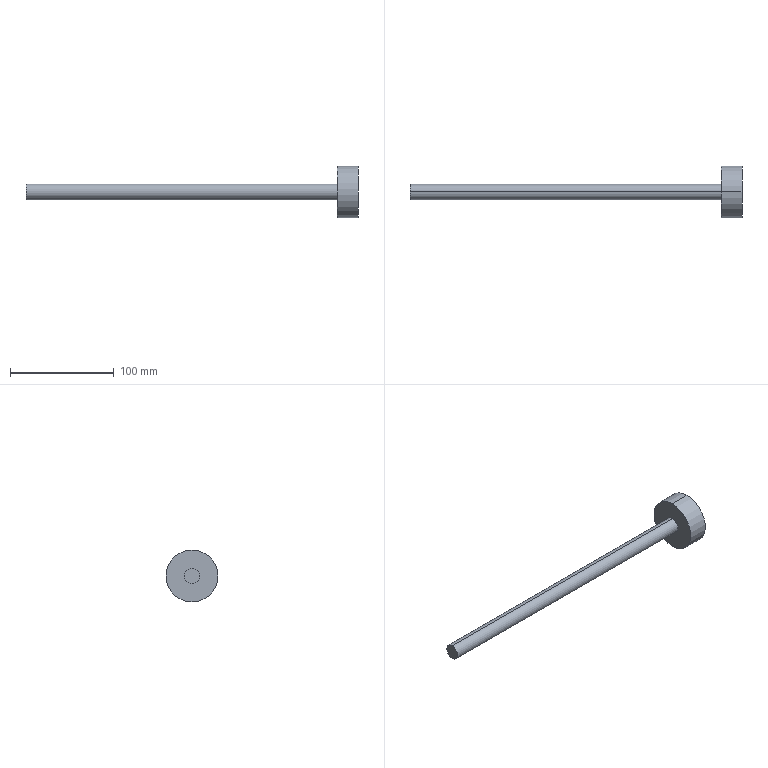Part | SolidWorks | features Revolution 1 | 1 solid | 7 faces | box 320 x 50 x 50 mm | volume 92284 mm3 | cylinder 4 | plane 3 | commonest cylinder face diameters 15 x2 50 x2
STEP:
#1=CARTESIAN_POINT('',(514.22,242.083,7.5));
#2=VERTEX_POINT('',#1);
#3=CARTESIAN_POINT('',(514.22,242.083,-7.5));
#4=VERTEX_POINT('',#3);
#5=CARTESIAN_POINT('',(514.22,242.083,0.));
#6=DIRECTION('',(-1.,0.,0.));
#7=DIRECTION('',(0.,0.,1.));
#8=AXIS2_PLACEMENT_3D('',#5,#6,#7);
#9=CIRCLE('',#8,7.5);
#10=EDGE_CURVE('',#2,#4,#9,.T.);
#11=ORIENTED_EDGE('',*,*,#10,.T.);
#12=CARTESIAN_POINT('',(214.22,242.083,-7.5));
#13=VERTEX_POINT('',#12);
#14=CARTESIAN_POINT('',(214.22,242.083,-7.5));
#15=DIRECTION('',(-1.,0.,0.));
#16=VECTOR('',#15,1000.);
#17=LINE('',#14,#16);
#18=EDGE_CURVE('',#4,#13,#17,.T.);
#19=ORIENTED_EDGE('',*,*,#18,.T.);
#20=CARTESIAN_POINT('',(214.22,242.083,7.5));
#21=VERTEX_POINT('',#20);
#22=CARTESIAN_POINT('',(214.22,242.083,0.));
#23=DIRECTION('',(-1.,0.,0.));
#24=DIRECTION('',(0.,0.,1.));
#25=AXIS2_PLACEMENT_3D('',#22,#23,#24);
#26=CIRCLE('',#25,7.5);
#27=EDGE_CURVE('',#21,#13,#26,.T.);
#28=ORIENTED_EDGE('',*,*,#27,.F.);
#29=CARTESIAN_POINT('',(214.22,242.083,7.5));
#30=DIRECTION('',(-1.,0.,0.));
#31=VECTOR('',#30,1000.);
#32=LINE('',#29,#31);
#33=EDGE_CURVE('',#2,#21,#32,.T.);
#34=ORIENTED_EDGE('',*,*,#33,.F.);
#35=EDGE_LOOP('',(#11,#19,#28,#34));
#36=FACE_OUTER_BOUND('',#35,.T.);
#37=CARTESIAN_POINT('',(214.22,242.083,0.));
#38=DIRECTION('',(-1.,0.,0.));
#39=DIRECTION('',(0.,0.,1.));
#40=AXIS2_PLACEMENT_3D('',#37,#38,#39);
#41=CYLINDRICAL_SURFACE('',#40,7.5);
#42=ADVANCED_FACE('',(#36),#41,.T.);
#43=CARTESIAN_POINT('',(534.22,242.083,25.));
#44=VERTEX_POINT('',#43);
#45=CARTESIAN_POINT('',(534.22,242.083,-25.));
#46=VERTEX_POINT('',#45);
#47=CARTESIAN_POINT('',(534.22,242.083,0.));
#48=DIRECTION('',(-1.,0.,0.));
#49=DIRECTION('',(0.,0.,1.));
#50=AXIS2_PLACEMENT_3D('',#47,#48,#49);
#51=CIRCLE('',#50,25.);
#52=EDGE_CURVE('',#44,#46,#51,.T.);
#53=ORIENTED_EDGE('',*,*,#52,.T.);
#54=CARTESIAN_POINT('',(514.22,242.083,-25.));
#55=VERTEX_POINT('',#54);
#56=CARTESIAN_POINT('',(214.22,242.083,-25.));
#57=DIRECTION('',(-1.,0.,0.));
#58=VECTOR('',#57,1000.);
#59=LINE('',#56,#58);
#60=EDGE_CURVE('',#46,#55,#59,.T.);
#61=ORIENTED_EDGE('',*,*,#60,.T.);
#62=CARTESIAN_POINT('',(514.22,242.083,25.));
#63=VERTEX_POINT('',#62);
#64=CARTESIAN_POINT('',(514.22,242.083,0.));
#65=DIRECTION('',(-1.,0.,0.));
#66=DIRECTION('',(0.,0.,1.));
#67=AXIS2_PLACEMENT_3D('',#64,#65,#66);
#68=CIRCLE('',#67,25.);
#69=EDGE_CURVE('',#63,#55,#68,.T.);
#70=ORIENTED_EDGE('',*,*,#69,.F.);
#71=CARTESIAN_POINT('',(214.22,242.083,25.));
#72=DIRECTION('',(-1.,0.,0.));
#73=VECTOR('',#72,1000.);
#74=LINE('',#71,#73);
#75=EDGE_CURVE('',#44,#63,#74,.T.);
#76=ORIENTED_EDGE('',*,*,#75,.F.);
#77=EDGE_LOOP('',(#53,#61,#70,#76));
#78=FACE_OUTER_BOUND('',#77,.T.);
#79=CARTESIAN_POINT('',(214.22,242.083,0.));
#80=DIRECTION('',(-1.,0.,0.));
#81=DIRECTION('',(0.,0.,1.));
#82=AXIS2_PLACEMENT_3D('',#79,#80,#81);
#83=CYLINDRICAL_SURFACE('',#82,25.);
#84=ADVANCED_FACE('',(#78),#83,.T.);
#85=ORIENTED_EDGE('',*,*,#27,.T.);
#86=CARTESIAN_POINT('',(214.22,242.083,0.));
#87=DIRECTION('',(-1.,0.,0.));
#88=DIRECTION('',(0.,0.,1.));
#89=AXIS2_PLACEMENT_3D('',#86,#87,#88);
#90=CIRCLE('',#89,7.5);
#91=EDGE_CURVE('',#13,#21,#90,.T.);
#92=ORIENTED_EDGE('',*,*,#91,.T.);
#93=EDGE_LOOP('',(#85,#92));
#94=FACE_OUTER_BOUND('',#93,.T.);
#95=CARTESIAN_POINT('',(214.22,249.583,0.));
#96=DIRECTION('',(1.,0.,0.));
#97=DIRECTION('',(0.,0.,-1.));
#98=AXIS2_PLACEMENT_3D('',#95,#96,#97);
#99=PLANE('',#98);
#100=ADVANCED_FACE('',(#94),#99,.F.);
#101=ORIENTED_EDGE('',*,*,#52,.F.);
#102=CARTESIAN_POINT('',(534.22,242.083,0.));
#103=DIRECTION('',(-1.,0.,0.));
#104=DIRECTION('',(0.,0.,1.));
#105=AXIS2_PLACEMENT_3D('',#102,#103,#104);
#106=CIRCLE('',#105,25.);
#107=EDGE_CURVE('',#46,#44,#106,.T.);
#108=ORIENTED_EDGE('',*,*,#107,.F.);
#109=EDGE_LOOP('',(#101,#108));
#110=FACE_OUTER_BOUND('',#109,.T.);
#111=CARTESIAN_POINT('',(534.22,242.083,0.));
#112=DIRECTION('',(-1.,0.,0.));
#113=DIRECTION('',(0.,0.,1.));
#114=AXIS2_PLACEMENT_3D('',#111,#112,#113);
#115=PLANE('',#114);
#116=ADVANCED_FACE('',(#110),#115,.F.);
#117=ORIENTED_EDGE('',*,*,#60,.F.);
#118=ORIENTED_EDGE('',*,*,#107,.T.);
#119=ORIENTED_EDGE('',*,*,#75,.T.);
#120=CARTESIAN_POINT('',(514.22,242.083,0.));
#121=DIRECTION('',(-1.,0.,0.));
#122=DIRECTION('',(0.,0.,1.));
#123=AXIS2_PLACEMENT_3D('',#120,#121,#122);
#124=CIRCLE('',#123,25.);
#125=EDGE_CURVE('',#55,#63,#124,.T.);
#126=ORIENTED_EDGE('',*,*,#125,.F.);
#127=EDGE_LOOP('',(#117,#118,#119,#126));
#128=FACE_OUTER_BOUND('',#127,.T.);
#129=CARTESIAN_POINT('',(214.22,242.083,0.));
#130=DIRECTION('',(-1.,0.,0.));
#131=DIRECTION('',(0.,0.,1.));
#132=AXIS2_PLACEMENT_3D('',#129,#130,#131);
#133=CYLINDRICAL_SURFACE('',#132,25.);
#134=ADVANCED_FACE('',(#128),#133,.T.);
#135=ORIENTED_EDGE('',*,*,#10,.F.);
#136=CARTESIAN_POINT('',(514.22,242.083,0.));
#137=DIRECTION('',(-1.,0.,0.));
#138=DIRECTION('',(0.,0.,1.));
#139=AXIS2_PLACEMENT_3D('',#136,#137,#138);
#140=CIRCLE('',#139,7.5);
#141=EDGE_CURVE('',#4,#2,#140,.T.);
#142=ORIENTED_EDGE('',*,*,#141,.F.);
#143=EDGE_LOOP('',(#135,#142));
#144=FACE_BOUND('',#143,.T.);
#145=ORIENTED_EDGE('',*,*,#69,.T.);
#146=ORIENTED_EDGE('',*,*,#125,.T.);
#147=EDGE_LOOP('',(#145,#146));
#148=FACE_OUTER_BOUND('',#147,.T.);
#149=CARTESIAN_POINT('',(514.22,267.083,0.));
#150=DIRECTION('',(1.,0.,0.));
#151=DIRECTION('',(0.,0.,-1.));
#152=AXIS2_PLACEMENT_3D('',#149,#150,#151);
#153=PLANE('',#152);
#154=ADVANCED_FACE('',(#144,#148),#153,.F.);
#155=ORIENTED_EDGE('',*,*,#18,.F.);
#156=ORIENTED_EDGE('',*,*,#141,.T.);
#157=ORIENTED_EDGE('',*,*,#33,.T.);
#158=ORIENTED_EDGE('',*,*,#91,.F.);
#159=EDGE_LOOP('',(#155,#156,#157,#158));
#160=FACE_OUTER_BOUND('',#159,.T.);
#161=CARTESIAN_POINT('',(214.22,242.083,0.));
#162=DIRECTION('',(-1.,0.,0.));
#163=DIRECTION('',(0.,0.,1.));
#164=AXIS2_PLACEMENT_3D('',#161,#162,#163);
#165=CYLINDRICAL_SURFACE('',#164,7.5);
#166=ADVANCED_FACE('',(#160),#165,.T.);
#167=CLOSED_SHELL('',(#42,#84,#100,#116,#134,#154,#166));
#168=MANIFOLD_SOLID_BREP('',#167);
#169=CARTESIAN_POINT('',(0.,0.,0.));
#170=DIRECTION('',(0.,0.,1.));
#171=DIRECTION('',(1.,0.,0.));
#172=AXIS2_PLACEMENT_3D('',#169,#170,#171);
#173=(LENGTH_UNIT()NAMED_UNIT(*)SI_UNIT(.MILLI.,.METRE.));
#174=UNCERTAINTY_MEASURE_WITH_UNIT(LENGTH_MEASURE(0.00001),#173,'','');
#175=(NAMED_UNIT(*)PLANE_ANGLE_UNIT()SI_UNIT($,.RADIAN.));
#176=(NAMED_UNIT(*)SI_UNIT($,.STERADIAN.)SOLID_ANGLE_UNIT());
#177=(GEOMETRIC_REPRESENTATION_CONTEXT(3)GLOBAL_UNCERTAINTY_ASSIGNED_CONTEXT((#174))GLOBAL_UNIT_ASSIGNED_CONTEXT((#173,#175,#176))REPRESENTATION_CONTEXT('',''));
#178=ADVANCED_BREP_SHAPE_REPRESENTATION('',(#168,#172),#177);